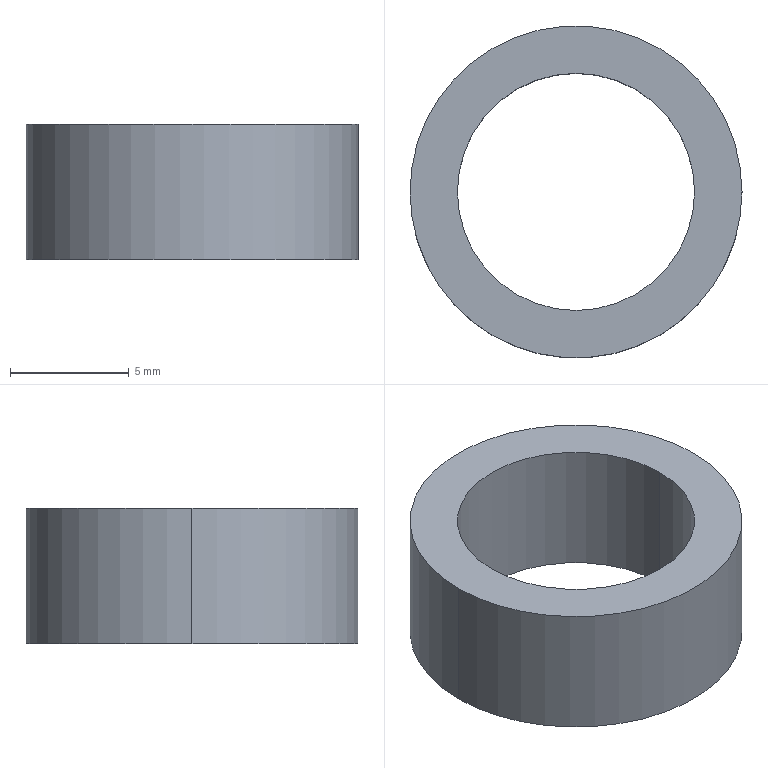Part | SolidWorks | features Extrusion 1 | 1 solid | 6 faces | box 14 x 14 x 5.7 mm | volume 429.77 mm3 | cylinder 4 | plane 2 | commonest cylinder face diameters 10 x2 14 x2
STEP:
#1=CARTESIAN_POINT('',(-5.,0.,5.7));
#2=VERTEX_POINT('',#1);
#3=CARTESIAN_POINT('',(5.,0.,5.7));
#4=VERTEX_POINT('',#3);
#5=CARTESIAN_POINT('',(0.,0.,5.7));
#6=DIRECTION('',(0.,0.,1.));
#7=DIRECTION('',(1.,0.,0.));
#8=AXIS2_PLACEMENT_3D('',#5,#6,#7);
#9=CIRCLE('',#8,5.);
#10=EDGE_CURVE('',#2,#4,#9,.T.);
#11=ORIENTED_EDGE('',*,*,#10,.T.);
#12=CARTESIAN_POINT('',(5.,0.,0.));
#13=VERTEX_POINT('',#12);
#14=CARTESIAN_POINT('',(5.,0.,5.7));
#15=DIRECTION('',(0.,0.,-1.));
#16=VECTOR('',#15,1000.);
#17=LINE('',#14,#16);
#18=EDGE_CURVE('',#4,#13,#17,.T.);
#19=ORIENTED_EDGE('',*,*,#18,.T.);
#20=CARTESIAN_POINT('',(-5.,0.,0.));
#21=VERTEX_POINT('',#20);
#22=CARTESIAN_POINT('',(0.,0.,0.));
#23=DIRECTION('',(0.,0.,1.));
#24=DIRECTION('',(1.,0.,0.));
#25=AXIS2_PLACEMENT_3D('',#22,#23,#24);
#26=CIRCLE('',#25,5.);
#27=EDGE_CURVE('',#21,#13,#26,.T.);
#28=ORIENTED_EDGE('',*,*,#27,.F.);
#29=CARTESIAN_POINT('',(-5.,0.,5.7));
#30=DIRECTION('',(0.,0.,-1.));
#31=VECTOR('',#30,1000.);
#32=LINE('',#29,#31);
#33=EDGE_CURVE('',#2,#21,#32,.T.);
#34=ORIENTED_EDGE('',*,*,#33,.F.);
#35=EDGE_LOOP('',(#11,#19,#28,#34));
#36=FACE_OUTER_BOUND('',#35,.T.);
#37=CARTESIAN_POINT('',(0.,0.,5.7));
#38=DIRECTION('',(0.,0.,-1.));
#39=DIRECTION('',(-1.,0.,0.));
#40=AXIS2_PLACEMENT_3D('',#37,#38,#39);
#41=CYLINDRICAL_SURFACE('',#40,5.);
#42=ADVANCED_FACE('',(#36),#41,.F.);
#43=CARTESIAN_POINT('',(7.,0.,5.7));
#44=VERTEX_POINT('',#43);
#45=CARTESIAN_POINT('',(-7.,0.,5.7));
#46=VERTEX_POINT('',#45);
#47=CARTESIAN_POINT('',(0.,0.,5.7));
#48=DIRECTION('',(0.,0.,1.));
#49=DIRECTION('',(1.,0.,0.));
#50=AXIS2_PLACEMENT_3D('',#47,#48,#49);
#51=CIRCLE('',#50,7.);
#52=EDGE_CURVE('',#44,#46,#51,.T.);
#53=ORIENTED_EDGE('',*,*,#52,.F.);
#54=CARTESIAN_POINT('',(7.,0.,0.));
#55=VERTEX_POINT('',#54);
#56=CARTESIAN_POINT('',(7.,0.,5.7));
#57=DIRECTION('',(0.,0.,-1.));
#58=VECTOR('',#57,1000.);
#59=LINE('',#56,#58);
#60=EDGE_CURVE('',#44,#55,#59,.T.);
#61=ORIENTED_EDGE('',*,*,#60,.T.);
#62=CARTESIAN_POINT('',(-7.,0.,0.));
#63=VERTEX_POINT('',#62);
#64=CARTESIAN_POINT('',(0.,0.,0.));
#65=DIRECTION('',(0.,0.,1.));
#66=DIRECTION('',(1.,0.,0.));
#67=AXIS2_PLACEMENT_3D('',#64,#65,#66);
#68=CIRCLE('',#67,7.);
#69=EDGE_CURVE('',#55,#63,#68,.T.);
#70=ORIENTED_EDGE('',*,*,#69,.T.);
#71=CARTESIAN_POINT('',(-7.,0.,5.7));
#72=DIRECTION('',(0.,0.,-1.));
#73=VECTOR('',#72,1000.);
#74=LINE('',#71,#73);
#75=EDGE_CURVE('',#46,#63,#74,.T.);
#76=ORIENTED_EDGE('',*,*,#75,.F.);
#77=EDGE_LOOP('',(#53,#61,#70,#76));
#78=FACE_OUTER_BOUND('',#77,.T.);
#79=CARTESIAN_POINT('',(0.,0.,5.7));
#80=DIRECTION('',(0.,0.,-1.));
#81=DIRECTION('',(-1.,0.,0.));
#82=AXIS2_PLACEMENT_3D('',#79,#80,#81);
#83=CYLINDRICAL_SURFACE('',#82,7.);
#84=ADVANCED_FACE('',(#78),#83,.T.);
#85=CARTESIAN_POINT('',(0.,0.,5.7));
#86=DIRECTION('',(0.,0.,1.));
#87=DIRECTION('',(1.,0.,0.));
#88=AXIS2_PLACEMENT_3D('',#85,#86,#87);
#89=CIRCLE('',#88,7.);
#90=EDGE_CURVE('',#46,#44,#89,.T.);
#91=ORIENTED_EDGE('',*,*,#90,.T.);
#92=ORIENTED_EDGE('',*,*,#52,.T.);
#93=EDGE_LOOP('',(#91,#92));
#94=FACE_OUTER_BOUND('',#93,.T.);
#95=ORIENTED_EDGE('',*,*,#10,.F.);
#96=CARTESIAN_POINT('',(0.,0.,5.7));
#97=DIRECTION('',(0.,0.,1.));
#98=DIRECTION('',(1.,0.,0.));
#99=AXIS2_PLACEMENT_3D('',#96,#97,#98);
#100=CIRCLE('',#99,5.);
#101=EDGE_CURVE('',#4,#2,#100,.T.);
#102=ORIENTED_EDGE('',*,*,#101,.F.);
#103=EDGE_LOOP('',(#95,#102));
#104=FACE_BOUND('',#103,.T.);
#105=CARTESIAN_POINT('',(0.,0.,5.7));
#106=DIRECTION('',(0.,0.,1.));
#107=DIRECTION('',(1.,0.,0.));
#108=AXIS2_PLACEMENT_3D('',#105,#106,#107);
#109=PLANE('',#108);
#110=ADVANCED_FACE('',(#94,#104),#109,.T.);
#111=CARTESIAN_POINT('',(0.,0.,0.));
#112=DIRECTION('',(0.,0.,1.));
#113=DIRECTION('',(1.,0.,0.));
#114=AXIS2_PLACEMENT_3D('',#111,#112,#113);
#115=CIRCLE('',#114,7.);
#116=EDGE_CURVE('',#63,#55,#115,.T.);
#117=ORIENTED_EDGE('',*,*,#116,.F.);
#118=ORIENTED_EDGE('',*,*,#69,.F.);
#119=EDGE_LOOP('',(#117,#118));
#120=FACE_OUTER_BOUND('',#119,.T.);
#121=ORIENTED_EDGE('',*,*,#27,.T.);
#122=CARTESIAN_POINT('',(0.,0.,0.));
#123=DIRECTION('',(0.,0.,1.));
#124=DIRECTION('',(1.,0.,0.));
#125=AXIS2_PLACEMENT_3D('',#122,#123,#124);
#126=CIRCLE('',#125,5.);
#127=EDGE_CURVE('',#13,#21,#126,.T.);
#128=ORIENTED_EDGE('',*,*,#127,.T.);
#129=EDGE_LOOP('',(#121,#128));
#130=FACE_BOUND('',#129,.T.);
#131=CARTESIAN_POINT('',(0.,0.,0.));
#132=DIRECTION('',(0.,0.,1.));
#133=DIRECTION('',(1.,0.,0.));
#134=AXIS2_PLACEMENT_3D('',#131,#132,#133);
#135=PLANE('',#134);
#136=ADVANCED_FACE('',(#120,#130),#135,.F.);
#137=ORIENTED_EDGE('',*,*,#60,.F.);
#138=ORIENTED_EDGE('',*,*,#90,.F.);
#139=ORIENTED_EDGE('',*,*,#75,.T.);
#140=ORIENTED_EDGE('',*,*,#116,.T.);
#141=EDGE_LOOP('',(#137,#138,#139,#140));
#142=FACE_OUTER_BOUND('',#141,.T.);
#143=CARTESIAN_POINT('',(0.,0.,5.7));
#144=DIRECTION('',(0.,0.,-1.));
#145=DIRECTION('',(-1.,0.,0.));
#146=AXIS2_PLACEMENT_3D('',#143,#144,#145);
#147=CYLINDRICAL_SURFACE('',#146,7.);
#148=ADVANCED_FACE('',(#142),#147,.T.);
#149=ORIENTED_EDGE('',*,*,#18,.F.);
#150=ORIENTED_EDGE('',*,*,#101,.T.);
#151=ORIENTED_EDGE('',*,*,#33,.T.);
#152=ORIENTED_EDGE('',*,*,#127,.F.);
#153=EDGE_LOOP('',(#149,#150,#151,#152));
#154=FACE_OUTER_BOUND('',#153,.T.);
#155=CARTESIAN_POINT('',(0.,0.,5.7));
#156=DIRECTION('',(0.,0.,-1.));
#157=DIRECTION('',(-1.,0.,0.));
#158=AXIS2_PLACEMENT_3D('',#155,#156,#157);
#159=CYLINDRICAL_SURFACE('',#158,5.);
#160=ADVANCED_FACE('',(#154),#159,.F.);
#161=CLOSED_SHELL('',(#42,#84,#110,#136,#148,#160));
#162=MANIFOLD_SOLID_BREP('',#161);
#163=CARTESIAN_POINT('',(0.,0.,0.));
#164=DIRECTION('',(0.,0.,1.));
#165=DIRECTION('',(1.,0.,0.));
#166=AXIS2_PLACEMENT_3D('',#163,#164,#165);
#167=(LENGTH_UNIT()NAMED_UNIT(*)SI_UNIT(.MILLI.,.METRE.));
#168=UNCERTAINTY_MEASURE_WITH_UNIT(LENGTH_MEASURE(0.00001),#167,'','');
#169=(NAMED_UNIT(*)PLANE_ANGLE_UNIT()SI_UNIT($,.RADIAN.));
#170=(NAMED_UNIT(*)SI_UNIT($,.STERADIAN.)SOLID_ANGLE_UNIT());
#171=(GEOMETRIC_REPRESENTATION_CONTEXT(3)GLOBAL_UNCERTAINTY_ASSIGNED_CONTEXT((#168))GLOBAL_UNIT_ASSIGNED_CONTEXT((#167,#169,#170))REPRESENTATION_CONTEXT('',''));
#172=ADVANCED_BREP_SHAPE_REPRESENTATION('',(#162,#166),#171);